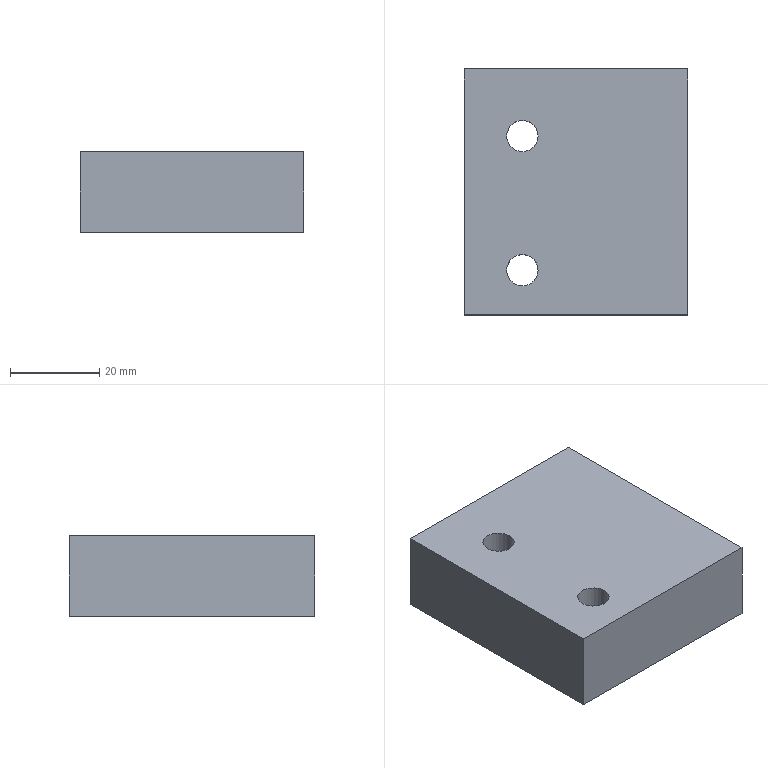Part | STEP file | lll_id674_x_t | 1 solid | 8 faces | box 50 x 55 x 18 mm | volume 48111 mm3 | plane 6 | cylinder 2 | commonest cylinder face diameters 7.009 x2
STEP:
#1=CARTESIAN_POINT('',(408.42,-87.5,-20.));
#2=VERTEX_POINT('',#1);
#3=CARTESIAN_POINT('',(408.42,-142.5,-20.));
#4=VERTEX_POINT('',#3);
#5=CARTESIAN_POINT('',(408.42,-87.5,-20.));
#6=DIRECTION('',(0.,-1.,0.));
#7=VECTOR('',#6,1.);
#8=LINE('',#5,#7);
#9=EDGE_CURVE('',#2,#4,#8,.T.);
#10=ORIENTED_EDGE('',*,*,#9,.T.);
#11=CARTESIAN_POINT('',(408.42,-142.5,-38.));
#12=VERTEX_POINT('',#11);
#13=CARTESIAN_POINT('',(408.42,-142.5,-38.));
#14=DIRECTION('',(0.,0.,1.));
#15=VECTOR('',#14,1.);
#16=LINE('',#13,#15);
#17=EDGE_CURVE('',#12,#4,#16,.T.);
#18=ORIENTED_EDGE('',*,*,#17,.F.);
#19=CARTESIAN_POINT('',(408.42,-87.5,-38.));
#20=VERTEX_POINT('',#19);
#21=CARTESIAN_POINT('',(408.42,-87.5,-38.));
#22=DIRECTION('',(0.,-1.,0.));
#23=VECTOR('',#22,1.);
#24=LINE('',#21,#23);
#25=EDGE_CURVE('',#20,#12,#24,.T.);
#26=ORIENTED_EDGE('',*,*,#25,.F.);
#27=CARTESIAN_POINT('',(408.42,-87.5,-38.));
#28=DIRECTION('',(0.,0.,1.));
#29=VECTOR('',#28,1.);
#30=LINE('',#27,#29);
#31=EDGE_CURVE('',#20,#2,#30,.T.);
#32=ORIENTED_EDGE('',*,*,#31,.T.);
#33=EDGE_LOOP('',(#10,#18,#26,#32));
#34=FACE_OUTER_BOUND('',#33,.T.);
#35=CARTESIAN_POINT('',(408.42,-87.5,-38.));
#36=DIRECTION('',(1.,0.,0.));
#37=DIRECTION('',(0.,0.,1.));
#38=AXIS2_PLACEMENT_3D('',#35,#36,#37);
#39=PLANE('',#38);
#40=ADVANCED_FACE('',(#34),#39,.T.);
#41=CARTESIAN_POINT('',(358.42,-142.5,-20.));
#42=VERTEX_POINT('',#41);
#43=CARTESIAN_POINT('',(408.42,-142.5,-20.));
#44=DIRECTION('',(-1.,0.,0.));
#45=VECTOR('',#44,1.);
#46=LINE('',#43,#45);
#47=EDGE_CURVE('',#4,#42,#46,.T.);
#48=ORIENTED_EDGE('',*,*,#47,.T.);
#49=CARTESIAN_POINT('',(358.42,-142.5,-38.));
#50=VERTEX_POINT('',#49);
#51=CARTESIAN_POINT('',(358.42,-142.5,-38.));
#52=DIRECTION('',(0.,0.,1.));
#53=VECTOR('',#52,1.);
#54=LINE('',#51,#53);
#55=EDGE_CURVE('',#50,#42,#54,.T.);
#56=ORIENTED_EDGE('',*,*,#55,.F.);
#57=CARTESIAN_POINT('',(408.42,-142.5,-38.));
#58=DIRECTION('',(-1.,0.,0.));
#59=VECTOR('',#58,1.);
#60=LINE('',#57,#59);
#61=EDGE_CURVE('',#12,#50,#60,.T.);
#62=ORIENTED_EDGE('',*,*,#61,.F.);
#63=ORIENTED_EDGE('',*,*,#17,.T.);
#64=EDGE_LOOP('',(#48,#56,#62,#63));
#65=FACE_OUTER_BOUND('',#64,.T.);
#66=CARTESIAN_POINT('',(408.42,-142.5,-38.));
#67=DIRECTION('',(0.,-1.,0.));
#68=DIRECTION('',(0.,0.,-1.));
#69=AXIS2_PLACEMENT_3D('',#66,#67,#68);
#70=PLANE('',#69);
#71=ADVANCED_FACE('',(#65),#70,.T.);
#72=CARTESIAN_POINT('',(358.42,-87.5,-20.));
#73=VERTEX_POINT('',#72);
#74=CARTESIAN_POINT('',(358.42,-142.5,-20.));
#75=DIRECTION('',(0.,1.,0.));
#76=VECTOR('',#75,1.);
#77=LINE('',#74,#76);
#78=EDGE_CURVE('',#42,#73,#77,.T.);
#79=ORIENTED_EDGE('',*,*,#78,.T.);
#80=CARTESIAN_POINT('',(358.42,-87.5,-38.));
#81=VERTEX_POINT('',#80);
#82=CARTESIAN_POINT('',(358.42,-87.5,-38.));
#83=DIRECTION('',(0.,0.,1.));
#84=VECTOR('',#83,1.);
#85=LINE('',#82,#84);
#86=EDGE_CURVE('',#81,#73,#85,.T.);
#87=ORIENTED_EDGE('',*,*,#86,.F.);
#88=CARTESIAN_POINT('',(358.42,-142.5,-38.));
#89=DIRECTION('',(0.,1.,0.));
#90=VECTOR('',#89,1.);
#91=LINE('',#88,#90);
#92=EDGE_CURVE('',#50,#81,#91,.T.);
#93=ORIENTED_EDGE('',*,*,#92,.F.);
#94=ORIENTED_EDGE('',*,*,#55,.T.);
#95=EDGE_LOOP('',(#79,#87,#93,#94));
#96=FACE_OUTER_BOUND('',#95,.T.);
#97=CARTESIAN_POINT('',(358.42,-142.5,-38.));
#98=DIRECTION('',(-1.,0.,0.));
#99=DIRECTION('',(0.,0.,-1.));
#100=AXIS2_PLACEMENT_3D('',#97,#98,#99);
#101=PLANE('',#100);
#102=ADVANCED_FACE('',(#96),#101,.T.);
#103=CARTESIAN_POINT('',(358.42,-87.5,-20.));
#104=DIRECTION('',(1.,0.,0.));
#105=VECTOR('',#104,1.);
#106=LINE('',#103,#105);
#107=EDGE_CURVE('',#73,#2,#106,.T.);
#108=ORIENTED_EDGE('',*,*,#107,.T.);
#109=ORIENTED_EDGE('',*,*,#31,.F.);
#110=CARTESIAN_POINT('',(358.42,-87.5,-38.));
#111=DIRECTION('',(1.,0.,0.));
#112=VECTOR('',#111,1.);
#113=LINE('',#110,#112);
#114=EDGE_CURVE('',#81,#20,#113,.T.);
#115=ORIENTED_EDGE('',*,*,#114,.F.);
#116=ORIENTED_EDGE('',*,*,#86,.T.);
#117=EDGE_LOOP('',(#108,#109,#115,#116));
#118=FACE_OUTER_BOUND('',#117,.T.);
#119=CARTESIAN_POINT('',(358.42,-87.5,-38.));
#120=DIRECTION('',(0.,1.,0.));
#121=DIRECTION('',(0.,0.,1.));
#122=AXIS2_PLACEMENT_3D('',#119,#120,#121);
#123=PLANE('',#122);
#124=ADVANCED_FACE('',(#118),#123,.T.);
#125=CARTESIAN_POINT('',(367.916,-132.5,-38.));
#126=VERTEX_POINT('',#125);
#127=CARTESIAN_POINT('',(371.42,-132.5,-38.));
#128=DIRECTION('',(0.,0.,1.));
#129=DIRECTION('',(-1.,0.,0.));
#130=AXIS2_PLACEMENT_3D('',#127,#128,#129);
#131=CIRCLE('',#130,3.505);
#132=EDGE_CURVE('',#126,#126,#131,.T.);
#133=ORIENTED_EDGE('',*,*,#132,.F.);
#134=EDGE_LOOP('',(#133));
#135=FACE_BOUND('',#134,.T.);
#136=CARTESIAN_POINT('',(367.916,-132.5,-20.));
#137=VERTEX_POINT('',#136);
#138=CARTESIAN_POINT('',(371.42,-132.5,-20.));
#139=DIRECTION('',(0.,0.,1.));
#140=DIRECTION('',(-1.,0.,0.));
#141=AXIS2_PLACEMENT_3D('',#138,#139,#140);
#142=CIRCLE('',#141,3.505);
#143=EDGE_CURVE('',#137,#137,#142,.T.);
#144=ORIENTED_EDGE('',*,*,#143,.T.);
#145=EDGE_LOOP('',(#144));
#146=FACE_BOUND('',#145,.T.);
#147=CARTESIAN_POINT('',(371.42,-132.5,-38.));
#148=DIRECTION('',(0.,0.,1.));
#149=DIRECTION('',(-1.,0.,0.));
#150=AXIS2_PLACEMENT_3D('',#147,#148,#149);
#151=CYLINDRICAL_SURFACE('',#150,3.505);
#152=ADVANCED_FACE('',(#135,#146),#151,.F.);
#153=CARTESIAN_POINT('',(367.916,-102.5,-38.));
#154=VERTEX_POINT('',#153);
#155=CARTESIAN_POINT('',(371.42,-102.5,-38.));
#156=DIRECTION('',(0.,0.,1.));
#157=DIRECTION('',(-1.,0.,0.));
#158=AXIS2_PLACEMENT_3D('',#155,#156,#157);
#159=CIRCLE('',#158,3.505);
#160=EDGE_CURVE('',#154,#154,#159,.T.);
#161=ORIENTED_EDGE('',*,*,#160,.F.);
#162=EDGE_LOOP('',(#161));
#163=FACE_BOUND('',#162,.T.);
#164=CARTESIAN_POINT('',(367.916,-102.5,-20.));
#165=VERTEX_POINT('',#164);
#166=CARTESIAN_POINT('',(371.42,-102.5,-20.));
#167=DIRECTION('',(0.,0.,1.));
#168=DIRECTION('',(-1.,0.,0.));
#169=AXIS2_PLACEMENT_3D('',#166,#167,#168);
#170=CIRCLE('',#169,3.505);
#171=EDGE_CURVE('',#165,#165,#170,.T.);
#172=ORIENTED_EDGE('',*,*,#171,.T.);
#173=EDGE_LOOP('',(#172));
#174=FACE_BOUND('',#173,.T.);
#175=CARTESIAN_POINT('',(371.42,-102.5,-38.));
#176=DIRECTION('',(0.,0.,1.));
#177=DIRECTION('',(-1.,0.,0.));
#178=AXIS2_PLACEMENT_3D('',#175,#176,#177);
#179=CYLINDRICAL_SURFACE('',#178,3.505);
#180=ADVANCED_FACE('',(#163,#174),#179,.F.);
#181=ORIENTED_EDGE('',*,*,#132,.T.);
#182=EDGE_LOOP('',(#181));
#183=FACE_BOUND('',#182,.T.);
#184=ORIENTED_EDGE('',*,*,#25,.T.);
#185=ORIENTED_EDGE('',*,*,#61,.T.);
#186=ORIENTED_EDGE('',*,*,#92,.T.);
#187=ORIENTED_EDGE('',*,*,#114,.T.);
#188=EDGE_LOOP('',(#184,#185,#186,#187));
#189=FACE_BOUND('',#188,.T.);
#190=ORIENTED_EDGE('',*,*,#160,.T.);
#191=EDGE_LOOP('',(#190));
#192=FACE_BOUND('',#191,.T.);
#193=CARTESIAN_POINT('',(0.,0.,-38.));
#194=DIRECTION('',(0.,0.,1.));
#195=DIRECTION('',(-1.,0.,0.));
#196=AXIS2_PLACEMENT_3D('',#193,#194,#195);
#197=PLANE('',#196);
#198=ADVANCED_FACE('',(#183,#189,#192),#197,.F.);
#199=ORIENTED_EDGE('',*,*,#143,.F.);
#200=EDGE_LOOP('',(#199));
#201=FACE_BOUND('',#200,.T.);
#202=ORIENTED_EDGE('',*,*,#9,.F.);
#203=ORIENTED_EDGE('',*,*,#107,.F.);
#204=ORIENTED_EDGE('',*,*,#78,.F.);
#205=ORIENTED_EDGE('',*,*,#47,.F.);
#206=EDGE_LOOP('',(#202,#203,#204,#205));
#207=FACE_BOUND('',#206,.T.);
#208=ORIENTED_EDGE('',*,*,#171,.F.);
#209=EDGE_LOOP('',(#208));
#210=FACE_BOUND('',#209,.T.);
#211=CARTESIAN_POINT('',(0.,0.,-20.));
#212=DIRECTION('',(0.,0.,1.));
#213=DIRECTION('',(-1.,0.,0.));
#214=AXIS2_PLACEMENT_3D('',#211,#212,#213);
#215=PLANE('',#214);
#216=ADVANCED_FACE('',(#201,#207,#210),#215,.T.);
#217=CLOSED_SHELL('',(#40,#71,#102,#124,#152,#180,#198,#216));
#218=MANIFOLD_SOLID_BREP('',#217);
#219=(LENGTH_UNIT()NAMED_UNIT(*)SI_UNIT(.MILLI.,.METRE.));
#220=UNCERTAINTY_MEASURE_WITH_UNIT(LENGTH_MEASURE(0.00002),#219,'','');
#221=(NAMED_UNIT(*)PLANE_ANGLE_UNIT()SI_UNIT($,.RADIAN.));
#222=PLANE_ANGLE_MEASURE_WITH_UNIT(PLANE_ANGLE_MEASURE(0.01745),#221);
#223=DIMENSIONAL_EXPONENTS(0.,0.,0.,0.,0.,0.,0.);
#224=(CONVERSION_BASED_UNIT('DEGREE',#222)NAMED_UNIT(#223)PLANE_ANGLE_UNIT());
#225=(NAMED_UNIT(*)SI_UNIT($,.STERADIAN.)SOLID_ANGLE_UNIT());
#226=(GEOMETRIC_REPRESENTATION_CONTEXT(3)GLOBAL_UNCERTAINTY_ASSIGNED_CONTEXT((#220))GLOBAL_UNIT_ASSIGNED_CONTEXT((#219,#224,#225))REPRESENTATION_CONTEXT('',''));
#227=ADVANCED_BREP_SHAPE_REPRESENTATION('',(#218),#226);